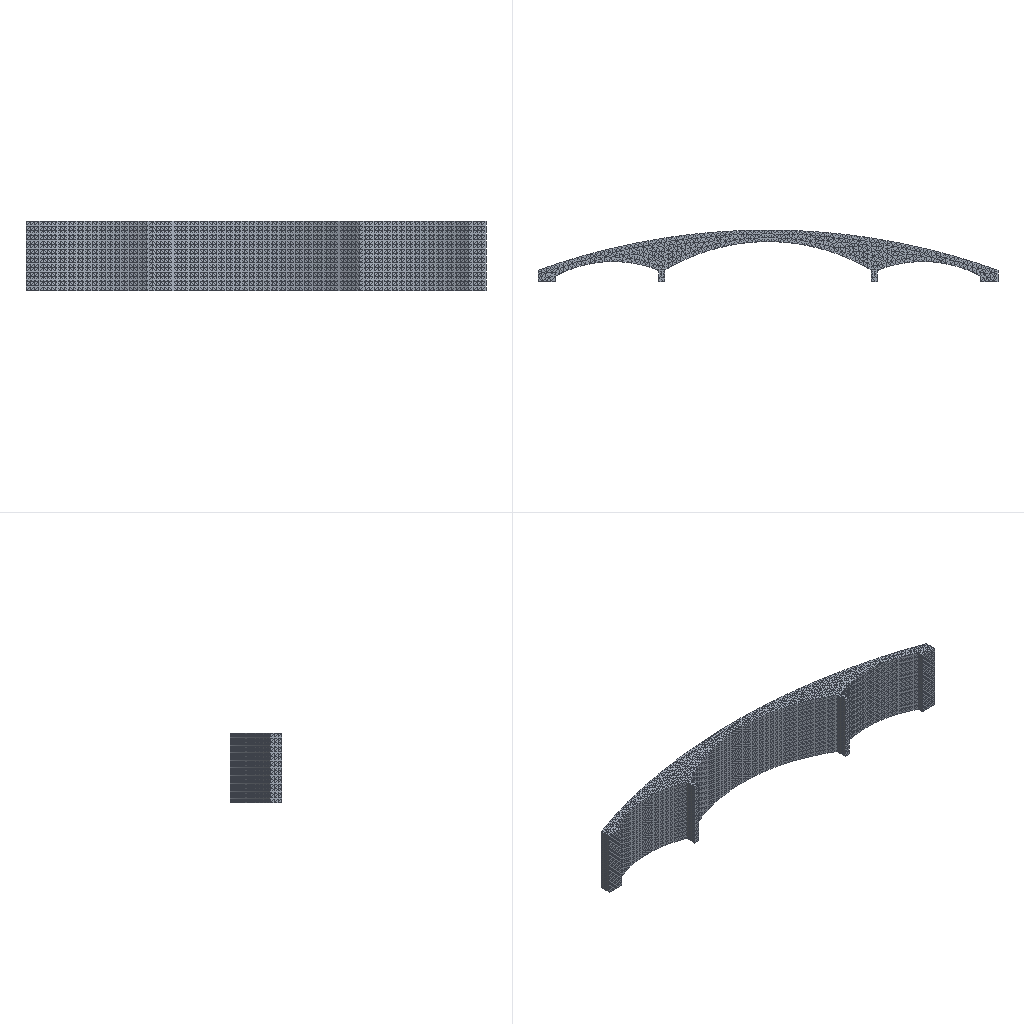Simulation study | abaqus
Set-up summary:
category,name,step,type,value,unit,region
solver,abaqus,,Abaqus/CAE 2024
units,unstated,,unstated,E=5.23e+07 density=2430 (no match)
analysis,Step-1,,frequency (modal),n_modes=30
mesh,nodes,,,57812
mesh,elements,,,36951
element_type,C3D10,,,36951
material,Material-1,,E,5.23e+07
material,Material-1,,nu,0.3
material,Material-1,,density,2430
section,Material-1,,solid section,,,Set-1
bc,BC-1,initial,fixed,"[dofs=rx,ry,rz,x,y,z n=6]",,Set-1
Abaqus input file, long lists of numbers shortened:
*Heading
** Job name: deck Model name: Model-1
** Generated by: Abaqus/CAE 2024
*Preprint, echo=NO, model=NO, history=NO, contact=NO
**
** PARTS
**
*Part, name=bridge
*Node
      1,          20.,           1.,           6.
      2,          20.,           0.,           6.
** (57810 more lines like these left out)
*Element, type=C3D10
    1,  4205,  4206,  4207,  4208,  8333,  8332,  8331,  8335,  8334,  8336
    2,  4205,  4206,  4209,  4210,  8333,  8338,  8337,  8340,  8339,  8341
** (36949 more lines like these left out)
*Nset, nset=Set-1, generate
     1,  57812,      1
*Elset, elset=Set-1, generate
     1,  36951,      1
** Section: Section-1
*Solid Section, elset=Set-1, material=Material-1
,
*End Part
**
**
** ASSEMBLY
**
*Assembly, name=Assembly
**
*Instance, name=bridge-1, part=bridge
*End Instance
**
*Nset, nset=Set-1, instance=bridge-1
     2,     3,     5,     6,     7,     8,     9,    10,    15,    16,    17,    18,    23,    24,    25,    26
    35,    36,    37,    38,    39,    40,    41,    42,    43,    44,    45,    46,    47,    48,    65,    66
** (45 more lines like these left out)
*Elset, elset=Set-1, instance=bridge-1
   259,  1586,  1911,  1916,  2301,  4185,  4848,  4927,  5139,  5202,  5559,  5562,  5580,  5581,  5590,  5609
  5634,  5642,  5656,  5663,  5697,  5699,  5702,  5723,  5742,  5747,  5752,  5760,  5841,  5849,  5856,  5867
** (17 more lines like these left out)
*End Assembly
**
** MATERIALS
**
*Material, name=Material-1
*Density
2430.,
*Elastic
 5.23e+07, 0.3
**
** BOUNDARY CONDITIONS
**
** Name: BC-1 Type: Displacement/Rotation
*Boundary
Set-1, 1, 1
Set-1, 2, 2
Set-1, 3, 3
Set-1, 4, 4
Set-1, 5, 5
Set-1, 6, 6
** ----------------------------------------------------------------
**
** STEP: Step-1
**
*Step, name=Step-1, nlgeom=NO, perturbation
*Frequency, eigensolver=Lanczos, sim=NO, acoustic coupling=on, normalization=displacement
30, , , , ,
**
** OUTPUT REQUESTS
**
*Restart, write, frequency=0
**
** FIELD OUTPUT: F-Output-1
**
*Output, field, variable=PRESELECT
*End Step
Results summary:
result,odb.job_status,,,JOB_STATUS_COMPLETED_SUCCESSFULLY,"consistent, unstated (Abaqus has no unit system)"
result,steps[0].procedure,Step-1,,*FREQUENCY,"consistent, unstated (Abaqus has no unit system)"
result,steps[0].time_period,Step-1,,0,"consistent, unstated (Abaqus has no unit system)"
result,steps[0].n_frames,Step-1,,31,"consistent, unstated (Abaqus has no unit system)"
result,steps[0].last_frame.id,Step-1,,1,"consistent, unstated (Abaqus has no unit system)"
result,steps[0].last_frame.value,Step-1,,30,"consistent, unstated (Abaqus has no unit system)"
result,steps[0].last_frame.description,Step-1,,Mode        30: Value =   1497.2     Freq =   6.158     (cycles/time),"consistent, unstated (Abaqus has no unit system)"
result,steps[0].max_U_magnitude,Step-1,,1.041,"consistent, unstated (Abaqus has no unit system)"
result,steps[0].eigenfrequencies_hz[1],Step-1,,0.8366,"consistent, unstated (Abaqus has no unit system)"
result,steps[0].eigenfrequencies_hz[2],Step-1,,0.9897,"consistent, unstated (Abaqus has no unit system)"
result,steps[0].eigenfrequencies_hz[3],Step-1,,1.24,"consistent, unstated (Abaqus has no unit system)"
result,steps[0].eigenfrequencies_hz[4],Step-1,,1.561,"consistent, unstated (Abaqus has no unit system)"
result,steps[0].eigenfrequencies_hz[5],Step-1,,1.688,"consistent, unstated (Abaqus has no unit system)"
result,steps[0].eigenfrequencies_hz[6],Step-1,,1.754,"consistent, unstated (Abaqus has no unit system)"
result,steps[0].eigenfrequencies_hz[7],Step-1,,1.885,"consistent, unstated (Abaqus has no unit system)"
result,steps[0].eigenfrequencies_hz[8],Step-1,,2.101,"consistent, unstated (Abaqus has no unit system)"
result,steps[0].eigenfrequencies_hz[9],Step-1,,2.258,"consistent, unstated (Abaqus has no unit system)"
result,steps[0].eigenfrequencies_hz[10],Step-1,,2.403,"consistent, unstated (Abaqus has no unit system)"
result,steps[0].eigenfrequencies_hz[11],Step-1,,2.576,"consistent, unstated (Abaqus has no unit system)"
result,steps[0].eigenfrequencies_hz[12],Step-1,,2.701,"consistent, unstated (Abaqus has no unit system)"
result,steps[0].eigenfrequencies_hz[13],Step-1,,2.909,"consistent, unstated (Abaqus has no unit system)"
result,steps[0].eigenfrequencies_hz[14],Step-1,,3.096,"consistent, unstated (Abaqus has no unit system)"
result,steps[0].eigenfrequencies_hz[15],Step-1,,3.157,"consistent, unstated (Abaqus has no unit system)"
result,steps[0].eigenfrequencies_hz[16],Step-1,,3.573,"consistent, unstated (Abaqus has no unit system)"
result,steps[0].eigenfrequencies_hz[17],Step-1,,3.647,"consistent, unstated (Abaqus has no unit system)"
result,steps[0].eigenfrequencies_hz[18],Step-1,,3.792,"consistent, unstated (Abaqus has no unit system)"
result,steps[0].eigenfrequencies_hz[19],Step-1,,3.864,"consistent, unstated (Abaqus has no unit system)"
result,steps[0].eigenfrequencies_hz[20],Step-1,,4.331,"consistent, unstated (Abaqus has no unit system)"
result,steps[0].eigenfrequencies_hz[21],Step-1,,4.355,"consistent, unstated (Abaqus has no unit system)"
result,steps[0].eigenfrequencies_hz[22],Step-1,,4.65,"consistent, unstated (Abaqus has no unit system)"
result,steps[0].eigenfrequencies_hz[23],Step-1,,5.092,"consistent, unstated (Abaqus has no unit system)"
result,steps[0].eigenfrequencies_hz[24],Step-1,,5.127,"consistent, unstated (Abaqus has no unit system)"
result,steps[0].eigenfrequencies_hz[25],Step-1,,5.153,"consistent, unstated (Abaqus has no unit system)"
result,steps[0].eigenfrequencies_hz[26],Step-1,,5.471,"consistent, unstated (Abaqus has no unit system)"
result,steps[0].eigenfrequencies_hz[27],Step-1,,5.526,"consistent, unstated (Abaqus has no unit system)"
result,steps[0].eigenfrequencies_hz[28],Step-1,,5.603,"consistent, unstated (Abaqus has no unit system)"
result,steps[0].eigenfrequencies_hz[29],Step-1,,5.604,"consistent, unstated (Abaqus has no unit system)"
result,steps[0].eigenfrequencies_hz[30],Step-1,,6.158,"consistent, unstated (Abaqus has no unit system)"
result,steps[0].diagnostic.n_increments,Step-1,,0,"consistent, unstated (Abaqus has no unit system)"